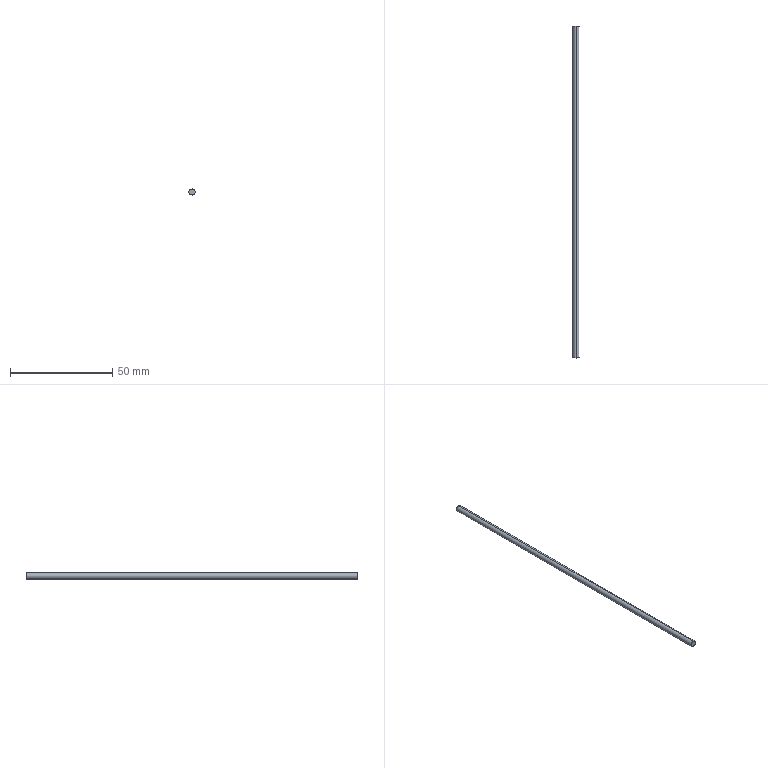Part | SolidWorks | features Extrusion 1 | 1 solid | 4 faces | box 3 x 162 x 3 mm | volume 1145 mm3 | cylinder 2 | plane 2 | commonest cylinder face diameters 3 x2
STEP:
#1=CARTESIAN_POINT('',(0.,162.,1.5));
#2=VERTEX_POINT('',#1);
#3=CARTESIAN_POINT('',(0.,162.,-1.5));
#4=VERTEX_POINT('',#3);
#5=CARTESIAN_POINT('',(0.,162.,0.));
#6=DIRECTION('',(0.,1.,0.));
#7=DIRECTION('',(0.,0.,1.));
#8=AXIS2_PLACEMENT_3D('',#5,#6,#7);
#9=CIRCLE('',#8,1.5);
#10=EDGE_CURVE('',#2,#4,#9,.T.);
#11=ORIENTED_EDGE('',*,*,#10,.F.);
#12=CARTESIAN_POINT('',(0.,0.,1.5));
#13=VERTEX_POINT('',#12);
#14=CARTESIAN_POINT('',(0.,162.,1.5));
#15=DIRECTION('',(0.,-1.,0.));
#16=VECTOR('',#15,1000.);
#17=LINE('',#14,#16);
#18=EDGE_CURVE('',#2,#13,#17,.T.);
#19=ORIENTED_EDGE('',*,*,#18,.T.);
#20=CARTESIAN_POINT('',(0.,0.,-1.5));
#21=VERTEX_POINT('',#20);
#22=CARTESIAN_POINT('',(0.,0.,0.));
#23=DIRECTION('',(0.,1.,0.));
#24=DIRECTION('',(0.,0.,1.));
#25=AXIS2_PLACEMENT_3D('',#22,#23,#24);
#26=CIRCLE('',#25,1.5);
#27=EDGE_CURVE('',#13,#21,#26,.T.);
#28=ORIENTED_EDGE('',*,*,#27,.T.);
#29=CARTESIAN_POINT('',(0.,162.,-1.5));
#30=DIRECTION('',(0.,-1.,0.));
#31=VECTOR('',#30,1000.);
#32=LINE('',#29,#31);
#33=EDGE_CURVE('',#4,#21,#32,.T.);
#34=ORIENTED_EDGE('',*,*,#33,.F.);
#35=EDGE_LOOP('',(#11,#19,#28,#34));
#36=FACE_OUTER_BOUND('',#35,.T.);
#37=CARTESIAN_POINT('',(0.,162.,0.));
#38=DIRECTION('',(0.,-1.,0.));
#39=DIRECTION('',(0.,0.,-1.));
#40=AXIS2_PLACEMENT_3D('',#37,#38,#39);
#41=CYLINDRICAL_SURFACE('',#40,1.5);
#42=ADVANCED_FACE('',(#36),#41,.T.);
#43=ORIENTED_EDGE('',*,*,#18,.F.);
#44=CARTESIAN_POINT('',(0.,162.,0.));
#45=DIRECTION('',(0.,1.,0.));
#46=DIRECTION('',(0.,0.,1.));
#47=AXIS2_PLACEMENT_3D('',#44,#45,#46);
#48=CIRCLE('',#47,1.5);
#49=EDGE_CURVE('',#4,#2,#48,.T.);
#50=ORIENTED_EDGE('',*,*,#49,.F.);
#51=ORIENTED_EDGE('',*,*,#33,.T.);
#52=CARTESIAN_POINT('',(0.,0.,0.));
#53=DIRECTION('',(0.,1.,0.));
#54=DIRECTION('',(0.,0.,1.));
#55=AXIS2_PLACEMENT_3D('',#52,#53,#54);
#56=CIRCLE('',#55,1.5);
#57=EDGE_CURVE('',#21,#13,#56,.T.);
#58=ORIENTED_EDGE('',*,*,#57,.T.);
#59=EDGE_LOOP('',(#43,#50,#51,#58));
#60=FACE_OUTER_BOUND('',#59,.T.);
#61=CARTESIAN_POINT('',(0.,162.,0.));
#62=DIRECTION('',(0.,-1.,0.));
#63=DIRECTION('',(0.,0.,-1.));
#64=AXIS2_PLACEMENT_3D('',#61,#62,#63);
#65=CYLINDRICAL_SURFACE('',#64,1.5);
#66=ADVANCED_FACE('',(#60),#65,.T.);
#67=ORIENTED_EDGE('',*,*,#49,.T.);
#68=ORIENTED_EDGE('',*,*,#10,.T.);
#69=EDGE_LOOP('',(#67,#68));
#70=FACE_OUTER_BOUND('',#69,.T.);
#71=CARTESIAN_POINT('',(0.,162.,0.));
#72=DIRECTION('',(0.,1.,0.));
#73=DIRECTION('',(0.,0.,1.));
#74=AXIS2_PLACEMENT_3D('',#71,#72,#73);
#75=PLANE('',#74);
#76=ADVANCED_FACE('',(#70),#75,.T.);
#77=ORIENTED_EDGE('',*,*,#57,.F.);
#78=ORIENTED_EDGE('',*,*,#27,.F.);
#79=EDGE_LOOP('',(#77,#78));
#80=FACE_OUTER_BOUND('',#79,.T.);
#81=CARTESIAN_POINT('',(0.,0.,0.));
#82=DIRECTION('',(0.,1.,0.));
#83=DIRECTION('',(0.,0.,1.));
#84=AXIS2_PLACEMENT_3D('',#81,#82,#83);
#85=PLANE('',#84);
#86=ADVANCED_FACE('',(#80),#85,.F.);
#87=CLOSED_SHELL('',(#42,#66,#76,#86));
#88=MANIFOLD_SOLID_BREP('',#87);
#89=CARTESIAN_POINT('',(0.,0.,0.));
#90=DIRECTION('',(0.,0.,1.));
#91=DIRECTION('',(1.,0.,0.));
#92=AXIS2_PLACEMENT_3D('',#89,#90,#91);
#93=(LENGTH_UNIT()NAMED_UNIT(*)SI_UNIT(.MILLI.,.METRE.));
#94=UNCERTAINTY_MEASURE_WITH_UNIT(LENGTH_MEASURE(0.00001),#93,'','');
#95=(NAMED_UNIT(*)PLANE_ANGLE_UNIT()SI_UNIT($,.RADIAN.));
#96=(NAMED_UNIT(*)SI_UNIT($,.STERADIAN.)SOLID_ANGLE_UNIT());
#97=(GEOMETRIC_REPRESENTATION_CONTEXT(3)GLOBAL_UNCERTAINTY_ASSIGNED_CONTEXT((#94))GLOBAL_UNIT_ASSIGNED_CONTEXT((#93,#95,#96))REPRESENTATION_CONTEXT('',''));
#98=ADVANCED_BREP_SHAPE_REPRESENTATION('',(#88,#92),#97);